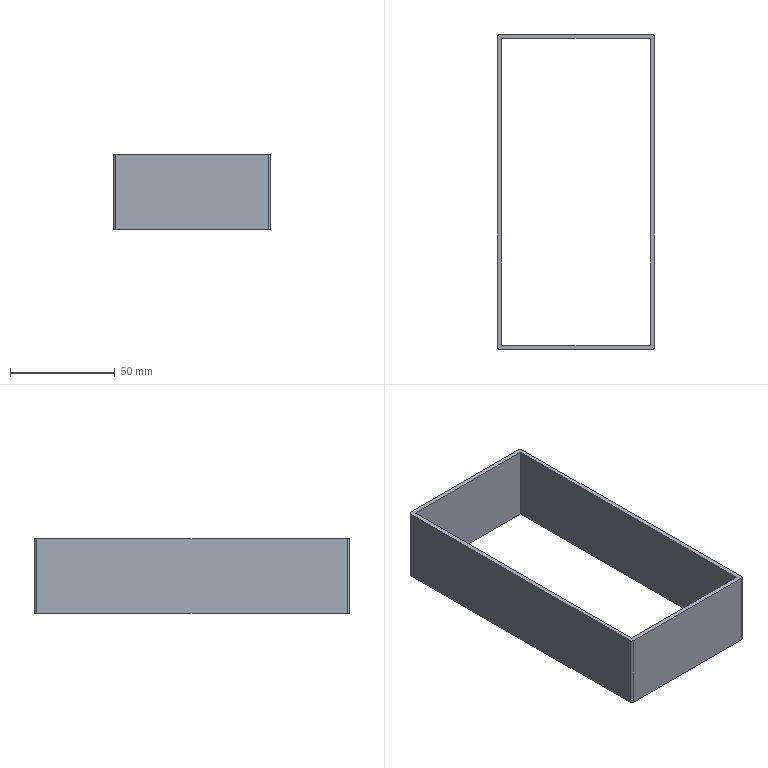Part | STEP file | 11 Timing Pulley盒 EDA50-R-011-BZ^EDA50-R04 (D60N) | 1 solid | 14 faces | box 75 x 150 x 36 mm | volume 31793 mm3 | plane 10 | cylinder 4 | commonest cylinder face diameters 2 x4
STEP:
#1=CARTESIAN_POINT('',(0.,0.,0.));
#2=DIRECTION('',(0.,0.,1.));
#3=DIRECTION('',(1.,0.,0.));
#4=AXIS2_PLACEMENT_3D('',#1,#2,#3);
#5=CARTESIAN_POINT('',(-37.5,113.,18.));
#6=VERTEX_POINT('',#5);
#7=CARTESIAN_POINT('',(-37.5,-35.,18.));
#8=VERTEX_POINT('',#7);
#9=CARTESIAN_POINT('',(-37.5,-36.,18.));
#10=DIRECTION('',(0.,-1.,0.));
#11=VECTOR('',#10,1.);
#12=LINE('',#9,#11);
#13=CARTESIAN_POINT('',(0.,0.,18.));
#14=DIRECTION('',(0.,0.,-1.));
#15=DIRECTION('',(-1.,0.,0.));
#16=AXIS2_PLACEMENT_3D('',#13,#14,#15);
#17=PLANE('',#16);
#18=CARTESIAN_POINT('',(37.5,-36.));
#19=DIRECTION('',(0.,-1.));
#20=VECTOR('',#19,1.);
#21=LINE('',#18,#20);
#22=(GEOMETRIC_REPRESENTATION_CONTEXT(2)PARAMETRIC_REPRESENTATION_CONTEXT()REPRESENTATION_CONTEXT('',''));
#23=DEFINITIONAL_REPRESENTATION('',(#21),#22);
#24=PCURVE('',#17,#23);
#25=CARTESIAN_POINT('',(-37.5,-36.,18.));
#26=DIRECTION('',(1.,0.,0.));
#27=DIRECTION('',(0.,0.,-1.));
#28=AXIS2_PLACEMENT_3D('',#25,#26,#27);
#29=PLANE('',#28);
#30=CARTESIAN_POINT('',(0.,0.));
#31=DIRECTION('',(0.,-1.));
#32=VECTOR('',#31,1.);
#33=LINE('',#30,#32);
#34=(GEOMETRIC_REPRESENTATION_CONTEXT(2)PARAMETRIC_REPRESENTATION_CONTEXT()REPRESENTATION_CONTEXT('',''));
#35=DEFINITIONAL_REPRESENTATION('',(#33),#34);
#36=PCURVE('',#29,#35);
#37=SURFACE_CURVE('',#12,(#24,#36),.PCURVE_S1.);
#38=EDGE_CURVE('',#6,#8,#37,.T.);
#39=ORIENTED_EDGE('',*,*,#38,.T.);
#40=CARTESIAN_POINT('',(-36.5,-36.,18.));
#41=VERTEX_POINT('',#40);
#42=CARTESIAN_POINT('',(-36.5,-35.,18.));
#43=DIRECTION('',(0.,0.,1.));
#44=DIRECTION('',(-1.,0.,0.));
#45=AXIS2_PLACEMENT_3D('',#42,#43,#44);
#46=CIRCLE('',#45,1.);
#47=CARTESIAN_POINT('',(37.5,-35.));
#48=CARTESIAN_POINT('',(37.5,-36.732));
#49=CARTESIAN_POINT('',(36.,-35.866));
#50=CARTESIAN_POINT('',(34.5,-35.));
#51=CARTESIAN_POINT('',(36.,-34.134));
#52=CARTESIAN_POINT('',(37.5,-33.268));
#53=CARTESIAN_POINT('',(37.5,-35.));
#54=(BOUNDED_CURVE()B_SPLINE_CURVE(2,(#47,#48,#49,#50,#51,#52,#53),.UNSPECIFIED.,.T.,.F.)B_SPLINE_CURVE_WITH_KNOTS((1,2,2,2,2,1),(-2.094,0.,2.094,4.189,6.283,8.378),.UNSPECIFIED.)CURVE()GEOMETRIC_REPRESENTATION_ITEM()RATIONAL_B_SPLINE_CURVE((1.,0.5,1.,0.5,1.,0.5,1.))REPRESENTATION_ITEM(''));
#55=(GEOMETRIC_REPRESENTATION_CONTEXT(2)PARAMETRIC_REPRESENTATION_CONTEXT()REPRESENTATION_CONTEXT('',''));
#56=DEFINITIONAL_REPRESENTATION('',(#54),#55);
#57=PCURVE('',#17,#56);
#58=CARTESIAN_POINT('',(-36.5,-35.,18.));
#59=DIRECTION('',(0.,0.,-1.));
#60=DIRECTION('',(-1.,0.,0.));
#61=AXIS2_PLACEMENT_3D('',#58,#59,#60);
#62=CYLINDRICAL_SURFACE('',#61,1.);
#63=CARTESIAN_POINT('',(6.283,0.));
#64=DIRECTION('',(-1.,0.));
#65=VECTOR('',#64,1.);
#66=LINE('',#63,#65);
#67=(GEOMETRIC_REPRESENTATION_CONTEXT(2)PARAMETRIC_REPRESENTATION_CONTEXT()REPRESENTATION_CONTEXT('',''));
#68=DEFINITIONAL_REPRESENTATION('',(#66),#67);
#69=PCURVE('',#62,#68);
#70=SURFACE_CURVE('',#46,(#57,#69),.PCURVE_S1.);
#71=EDGE_CURVE('',#8,#41,#70,.T.);
#72=ORIENTED_EDGE('',*,*,#71,.T.);
#73=CARTESIAN_POINT('',(36.5,-36.,18.));
#74=VERTEX_POINT('',#73);
#75=CARTESIAN_POINT('',(-37.5,-36.,18.));
#76=DIRECTION('',(1.,0.,0.));
#77=VECTOR('',#76,1.);
#78=LINE('',#75,#77);
#79=CARTESIAN_POINT('',(37.5,-36.));
#80=DIRECTION('',(-1.,0.));
#81=VECTOR('',#80,1.);
#82=LINE('',#79,#81);
#83=(GEOMETRIC_REPRESENTATION_CONTEXT(2)PARAMETRIC_REPRESENTATION_CONTEXT()REPRESENTATION_CONTEXT('',''));
#84=DEFINITIONAL_REPRESENTATION('',(#82),#83);
#85=PCURVE('',#17,#84);
#86=CARTESIAN_POINT('',(-37.5,-36.,18.));
#87=DIRECTION('',(0.,1.,0.));
#88=DIRECTION('',(0.,0.,1.));
#89=AXIS2_PLACEMENT_3D('',#86,#87,#88);
#90=PLANE('',#89);
#91=CARTESIAN_POINT('',(0.,0.));
#92=DIRECTION('',(0.,1.));
#93=VECTOR('',#92,1.);
#94=LINE('',#91,#93);
#95=(GEOMETRIC_REPRESENTATION_CONTEXT(2)PARAMETRIC_REPRESENTATION_CONTEXT()REPRESENTATION_CONTEXT('',''));
#96=DEFINITIONAL_REPRESENTATION('',(#94),#95);
#97=PCURVE('',#90,#96);
#98=SURFACE_CURVE('',#78,(#85,#97),.PCURVE_S1.);
#99=EDGE_CURVE('',#41,#74,#98,.T.);
#100=ORIENTED_EDGE('',*,*,#99,.T.);
#101=CARTESIAN_POINT('',(37.5,-35.,18.));
#102=VERTEX_POINT('',#101);
#103=CARTESIAN_POINT('',(36.5,-35.,18.));
#104=DIRECTION('',(0.,0.,1.));
#105=DIRECTION('',(-1.,0.,0.));
#106=AXIS2_PLACEMENT_3D('',#103,#104,#105);
#107=CIRCLE('',#106,1.);
#108=CARTESIAN_POINT('',(-35.5,-35.));
#109=CARTESIAN_POINT('',(-35.5,-36.732));
#110=CARTESIAN_POINT('',(-37.,-35.866));
#111=CARTESIAN_POINT('',(-38.5,-35.));
#112=CARTESIAN_POINT('',(-37.,-34.134));
#113=CARTESIAN_POINT('',(-35.5,-33.268));
#114=CARTESIAN_POINT('',(-35.5,-35.));
#115=(BOUNDED_CURVE()B_SPLINE_CURVE(2,(#108,#109,#110,#111,#112,#113,#114),.UNSPECIFIED.,.T.,.F.)B_SPLINE_CURVE_WITH_KNOTS((1,2,2,2,2,1),(-2.094,0.,2.094,4.189,6.283,8.378),.UNSPECIFIED.)CURVE()GEOMETRIC_REPRESENTATION_ITEM()RATIONAL_B_SPLINE_CURVE((1.,0.5,1.,0.5,1.,0.5,1.))REPRESENTATION_ITEM(''));
#116=(GEOMETRIC_REPRESENTATION_CONTEXT(2)PARAMETRIC_REPRESENTATION_CONTEXT()REPRESENTATION_CONTEXT('',''));
#117=DEFINITIONAL_REPRESENTATION('',(#115),#116);
#118=PCURVE('',#17,#117);
#119=CARTESIAN_POINT('',(36.5,-35.,18.));
#120=DIRECTION('',(0.,0.,-1.));
#121=DIRECTION('',(-1.,0.,0.));
#122=AXIS2_PLACEMENT_3D('',#119,#120,#121);
#123=CYLINDRICAL_SURFACE('',#122,1.);
#124=CARTESIAN_POINT('',(6.283,0.));
#125=DIRECTION('',(-1.,0.));
#126=VECTOR('',#125,1.);
#127=LINE('',#124,#126);
#128=(GEOMETRIC_REPRESENTATION_CONTEXT(2)PARAMETRIC_REPRESENTATION_CONTEXT()REPRESENTATION_CONTEXT('',''));
#129=DEFINITIONAL_REPRESENTATION('',(#127),#128);
#130=PCURVE('',#123,#129);
#131=SURFACE_CURVE('',#107,(#118,#130),.PCURVE_S1.);
#132=EDGE_CURVE('',#74,#102,#131,.T.);
#133=ORIENTED_EDGE('',*,*,#132,.T.);
#134=CARTESIAN_POINT('',(37.5,113.,18.));
#135=VERTEX_POINT('',#134);
#136=CARTESIAN_POINT('',(37.5,-36.,18.));
#137=DIRECTION('',(0.,1.,0.));
#138=VECTOR('',#137,1.);
#139=LINE('',#136,#138);
#140=CARTESIAN_POINT('',(-37.5,-36.));
#141=DIRECTION('',(0.,1.));
#142=VECTOR('',#141,1.);
#143=LINE('',#140,#142);
#144=(GEOMETRIC_REPRESENTATION_CONTEXT(2)PARAMETRIC_REPRESENTATION_CONTEXT()REPRESENTATION_CONTEXT('',''));
#145=DEFINITIONAL_REPRESENTATION('',(#143),#144);
#146=PCURVE('',#17,#145);
#147=CARTESIAN_POINT('',(37.5,-36.,18.));
#148=DIRECTION('',(-1.,0.,0.));
#149=DIRECTION('',(0.,0.,1.));
#150=AXIS2_PLACEMENT_3D('',#147,#148,#149);
#151=PLANE('',#150);
#152=CARTESIAN_POINT('',(0.,0.));
#153=DIRECTION('',(0.,1.));
#154=VECTOR('',#153,1.);
#155=LINE('',#152,#154);
#156=(GEOMETRIC_REPRESENTATION_CONTEXT(2)PARAMETRIC_REPRESENTATION_CONTEXT()REPRESENTATION_CONTEXT('',''));
#157=DEFINITIONAL_REPRESENTATION('',(#155),#156);
#158=PCURVE('',#151,#157);
#159=SURFACE_CURVE('',#139,(#146,#158),.PCURVE_S1.);
#160=EDGE_CURVE('',#102,#135,#159,.T.);
#161=ORIENTED_EDGE('',*,*,#160,.T.);
#162=CARTESIAN_POINT('',(36.5,114.,18.));
#163=VERTEX_POINT('',#162);
#164=CARTESIAN_POINT('',(36.5,113.,18.));
#165=DIRECTION('',(0.,0.,1.));
#166=DIRECTION('',(-1.,0.,0.));
#167=AXIS2_PLACEMENT_3D('',#164,#165,#166);
#168=CIRCLE('',#167,1.);
#169=CARTESIAN_POINT('',(-35.5,113.));
#170=CARTESIAN_POINT('',(-35.5,111.268));
#171=CARTESIAN_POINT('',(-37.,112.134));
#172=CARTESIAN_POINT('',(-38.5,113.));
#173=CARTESIAN_POINT('',(-37.,113.866));
#174=CARTESIAN_POINT('',(-35.5,114.732));
#175=CARTESIAN_POINT('',(-35.5,113.));
#176=(BOUNDED_CURVE()B_SPLINE_CURVE(2,(#169,#170,#171,#172,#173,#174,#175),.UNSPECIFIED.,.T.,.F.)B_SPLINE_CURVE_WITH_KNOTS((1,2,2,2,2,1),(-2.094,0.,2.094,4.189,6.283,8.378),.UNSPECIFIED.)CURVE()GEOMETRIC_REPRESENTATION_ITEM()RATIONAL_B_SPLINE_CURVE((1.,0.5,1.,0.5,1.,0.5,1.))REPRESENTATION_ITEM(''));
#177=(GEOMETRIC_REPRESENTATION_CONTEXT(2)PARAMETRIC_REPRESENTATION_CONTEXT()REPRESENTATION_CONTEXT('',''));
#178=DEFINITIONAL_REPRESENTATION('',(#176),#177);
#179=PCURVE('',#17,#178);
#180=CARTESIAN_POINT('',(36.5,113.,18.));
#181=DIRECTION('',(0.,0.,-1.));
#182=DIRECTION('',(-1.,0.,0.));
#183=AXIS2_PLACEMENT_3D('',#180,#181,#182);
#184=CYLINDRICAL_SURFACE('',#183,1.);
#185=CARTESIAN_POINT('',(6.283,0.));
#186=DIRECTION('',(-1.,0.));
#187=VECTOR('',#186,1.);
#188=LINE('',#185,#187);
#189=(GEOMETRIC_REPRESENTATION_CONTEXT(2)PARAMETRIC_REPRESENTATION_CONTEXT()REPRESENTATION_CONTEXT('',''));
#190=DEFINITIONAL_REPRESENTATION('',(#188),#189);
#191=PCURVE('',#184,#190);
#192=SURFACE_CURVE('',#168,(#179,#191),.PCURVE_S1.);
#193=EDGE_CURVE('',#135,#163,#192,.T.);
#194=ORIENTED_EDGE('',*,*,#193,.T.);
#195=CARTESIAN_POINT('',(-36.5,114.,18.));
#196=VERTEX_POINT('',#195);
#197=CARTESIAN_POINT('',(-37.5,114.,18.));
#198=DIRECTION('',(-1.,0.,0.));
#199=VECTOR('',#198,1.);
#200=LINE('',#197,#199);
#201=CARTESIAN_POINT('',(37.5,114.));
#202=DIRECTION('',(1.,0.));
#203=VECTOR('',#202,1.);
#204=LINE('',#201,#203);
#205=(GEOMETRIC_REPRESENTATION_CONTEXT(2)PARAMETRIC_REPRESENTATION_CONTEXT()REPRESENTATION_CONTEXT('',''));
#206=DEFINITIONAL_REPRESENTATION('',(#204),#205);
#207=PCURVE('',#17,#206);
#208=CARTESIAN_POINT('',(-37.5,114.,18.));
#209=DIRECTION('',(0.,-1.,0.));
#210=DIRECTION('',(0.,0.,-1.));
#211=AXIS2_PLACEMENT_3D('',#208,#209,#210);
#212=PLANE('',#211);
#213=CARTESIAN_POINT('',(0.,0.));
#214=DIRECTION('',(0.,-1.));
#215=VECTOR('',#214,1.);
#216=LINE('',#213,#215);
#217=(GEOMETRIC_REPRESENTATION_CONTEXT(2)PARAMETRIC_REPRESENTATION_CONTEXT()REPRESENTATION_CONTEXT('',''));
#218=DEFINITIONAL_REPRESENTATION('',(#216),#217);
#219=PCURVE('',#212,#218);
#220=SURFACE_CURVE('',#200,(#207,#219),.PCURVE_S1.);
#221=EDGE_CURVE('',#163,#196,#220,.T.);
#222=ORIENTED_EDGE('',*,*,#221,.T.);
#223=CARTESIAN_POINT('',(-36.5,113.,18.));
#224=DIRECTION('',(0.,0.,1.));
#225=DIRECTION('',(-1.,0.,0.));
#226=AXIS2_PLACEMENT_3D('',#223,#224,#225);
#227=CIRCLE('',#226,1.);
#228=CARTESIAN_POINT('',(37.5,113.));
#229=CARTESIAN_POINT('',(37.5,111.268));
#230=CARTESIAN_POINT('',(36.,112.134));
#231=CARTESIAN_POINT('',(34.5,113.));
#232=CARTESIAN_POINT('',(36.,113.866));
#233=CARTESIAN_POINT('',(37.5,114.732));
#234=CARTESIAN_POINT('',(37.5,113.));
#235=(BOUNDED_CURVE()B_SPLINE_CURVE(2,(#228,#229,#230,#231,#232,#233,#234),.UNSPECIFIED.,.T.,.F.)B_SPLINE_CURVE_WITH_KNOTS((1,2,2,2,2,1),(-2.094,0.,2.094,4.189,6.283,8.378),.UNSPECIFIED.)CURVE()GEOMETRIC_REPRESENTATION_ITEM()RATIONAL_B_SPLINE_CURVE((1.,0.5,1.,0.5,1.,0.5,1.))REPRESENTATION_ITEM(''));
#236=(GEOMETRIC_REPRESENTATION_CONTEXT(2)PARAMETRIC_REPRESENTATION_CONTEXT()REPRESENTATION_CONTEXT('',''));
#237=DEFINITIONAL_REPRESENTATION('',(#235),#236);
#238=PCURVE('',#17,#237);
#239=CARTESIAN_POINT('',(-36.5,113.,18.));
#240=DIRECTION('',(0.,0.,-1.));
#241=DIRECTION('',(-1.,0.,0.));
#242=AXIS2_PLACEMENT_3D('',#239,#240,#241);
#243=CYLINDRICAL_SURFACE('',#242,1.);
#244=CARTESIAN_POINT('',(6.283,0.));
#245=DIRECTION('',(-1.,0.));
#246=VECTOR('',#245,1.);
#247=LINE('',#244,#246);
#248=(GEOMETRIC_REPRESENTATION_CONTEXT(2)PARAMETRIC_REPRESENTATION_CONTEXT()REPRESENTATION_CONTEXT('',''));
#249=DEFINITIONAL_REPRESENTATION('',(#247),#248);
#250=PCURVE('',#243,#249);
#251=SURFACE_CURVE('',#227,(#238,#250),.PCURVE_S1.);
#252=EDGE_CURVE('',#196,#6,#251,.T.);
#253=ORIENTED_EDGE('',*,*,#252,.T.);
#254=EDGE_LOOP('',(#39,#72,#100,#133,#161,#194,#222,#253));
#255=FACE_BOUND('',#254,.T.);
#256=CARTESIAN_POINT('',(-35.5,112.,18.));
#257=VERTEX_POINT('',#256);
#258=CARTESIAN_POINT('',(-35.5,-34.,18.));
#259=VERTEX_POINT('',#258);
#260=CARTESIAN_POINT('',(-35.5,-34.,18.));
#261=DIRECTION('',(0.,-1.,0.));
#262=VECTOR('',#261,1.);
#263=LINE('',#260,#262);
#264=CARTESIAN_POINT('',(35.5,-34.));
#265=DIRECTION('',(0.,-1.));
#266=VECTOR('',#265,1.);
#267=LINE('',#264,#266);
#268=(GEOMETRIC_REPRESENTATION_CONTEXT(2)PARAMETRIC_REPRESENTATION_CONTEXT()REPRESENTATION_CONTEXT('',''));
#269=DEFINITIONAL_REPRESENTATION('',(#267),#268);
#270=PCURVE('',#17,#269);
#271=CARTESIAN_POINT('',(-35.5,-34.,18.));
#272=DIRECTION('',(1.,0.,0.));
#273=DIRECTION('',(0.,0.,-1.));
#274=AXIS2_PLACEMENT_3D('',#271,#272,#273);
#275=PLANE('',#274);
#276=CARTESIAN_POINT('',(0.,0.));
#277=DIRECTION('',(0.,-1.));
#278=VECTOR('',#277,1.);
#279=LINE('',#276,#278);
#280=(GEOMETRIC_REPRESENTATION_CONTEXT(2)PARAMETRIC_REPRESENTATION_CONTEXT()REPRESENTATION_CONTEXT('',''));
#281=DEFINITIONAL_REPRESENTATION('',(#279),#280);
#282=PCURVE('',#275,#281);
#283=SURFACE_CURVE('',#263,(#270,#282),.PCURVE_S1.);
#284=EDGE_CURVE('',#257,#259,#283,.T.);
#285=ORIENTED_EDGE('',*,*,#284,.F.);
#286=CARTESIAN_POINT('',(35.5,112.,18.));
#287=VERTEX_POINT('',#286);
#288=CARTESIAN_POINT('',(-35.5,112.,18.));
#289=DIRECTION('',(-1.,0.,0.));
#290=VECTOR('',#289,1.);
#291=LINE('',#288,#290);
#292=CARTESIAN_POINT('',(35.5,112.));
#293=DIRECTION('',(1.,0.));
#294=VECTOR('',#293,1.);
#295=LINE('',#292,#294);
#296=(GEOMETRIC_REPRESENTATION_CONTEXT(2)PARAMETRIC_REPRESENTATION_CONTEXT()REPRESENTATION_CONTEXT('',''));
#297=DEFINITIONAL_REPRESENTATION('',(#295),#296);
#298=PCURVE('',#17,#297);
#299=CARTESIAN_POINT('',(-35.5,112.,18.));
#300=DIRECTION('',(0.,-1.,0.));
#301=DIRECTION('',(0.,0.,-1.));
#302=AXIS2_PLACEMENT_3D('',#299,#300,#301);
#303=PLANE('',#302);
#304=CARTESIAN_POINT('',(0.,0.));
#305=DIRECTION('',(0.,-1.));
#306=VECTOR('',#305,1.);
#307=LINE('',#304,#306);
#308=(GEOMETRIC_REPRESENTATION_CONTEXT(2)PARAMETRIC_REPRESENTATION_CONTEXT()REPRESENTATION_CONTEXT('',''));
#309=DEFINITIONAL_REPRESENTATION('',(#307),#308);
#310=PCURVE('',#303,#309);
#311=SURFACE_CURVE('',#291,(#298,#310),.PCURVE_S1.);
#312=EDGE_CURVE('',#287,#257,#311,.T.);
#313=ORIENTED_EDGE('',*,*,#312,.F.);
#314=CARTESIAN_POINT('',(35.5,-34.,18.));
#315=VERTEX_POINT('',#314);
#316=CARTESIAN_POINT('',(35.5,-34.,18.));
#317=DIRECTION('',(0.,1.,0.));
#318=VECTOR('',#317,1.);
#319=LINE('',#316,#318);
#320=CARTESIAN_POINT('',(-35.5,-34.));
#321=DIRECTION('',(0.,1.));
#322=VECTOR('',#321,1.);
#323=LINE('',#320,#322);
#324=(GEOMETRIC_REPRESENTATION_CONTEXT(2)PARAMETRIC_REPRESENTATION_CONTEXT()REPRESENTATION_CONTEXT('',''));
#325=DEFINITIONAL_REPRESENTATION('',(#323),#324);
#326=PCURVE('',#17,#325);
#327=CARTESIAN_POINT('',(35.5,-34.,18.));
#328=DIRECTION('',(-1.,0.,0.));
#329=DIRECTION('',(0.,0.,1.));
#330=AXIS2_PLACEMENT_3D('',#327,#328,#329);
#331=PLANE('',#330);
#332=CARTESIAN_POINT('',(0.,0.));
#333=DIRECTION('',(0.,1.));
#334=VECTOR('',#333,1.);
#335=LINE('',#332,#334);
#336=(GEOMETRIC_REPRESENTATION_CONTEXT(2)PARAMETRIC_REPRESENTATION_CONTEXT()REPRESENTATION_CONTEXT('',''));
#337=DEFINITIONAL_REPRESENTATION('',(#335),#336);
#338=PCURVE('',#331,#337);
#339=SURFACE_CURVE('',#319,(#326,#338),.PCURVE_S1.);
#340=EDGE_CURVE('',#315,#287,#339,.T.);
#341=ORIENTED_EDGE('',*,*,#340,.F.);
#342=CARTESIAN_POINT('',(-35.5,-34.,18.));
#343=DIRECTION('',(1.,0.,0.));
#344=VECTOR('',#343,1.);
#345=LINE('',#342,#344);
#346=CARTESIAN_POINT('',(35.5,-34.));
#347=DIRECTION('',(-1.,0.));
#348=VECTOR('',#347,1.);
#349=LINE('',#346,#348);
#350=(GEOMETRIC_REPRESENTATION_CONTEXT(2)PARAMETRIC_REPRESENTATION_CONTEXT()REPRESENTATION_CONTEXT('',''));
#351=DEFINITIONAL_REPRESENTATION('',(#349),#350);
#352=PCURVE('',#17,#351);
#353=CARTESIAN_POINT('',(-35.5,-34.,18.));
#354=DIRECTION('',(0.,1.,0.));
#355=DIRECTION('',(0.,0.,1.));
#356=AXIS2_PLACEMENT_3D('',#353,#354,#355);
#357=PLANE('',#356);
#358=CARTESIAN_POINT('',(0.,0.));
#359=DIRECTION('',(0.,1.));
#360=VECTOR('',#359,1.);
#361=LINE('',#358,#360);
#362=(GEOMETRIC_REPRESENTATION_CONTEXT(2)PARAMETRIC_REPRESENTATION_CONTEXT()REPRESENTATION_CONTEXT('',''));
#363=DEFINITIONAL_REPRESENTATION('',(#361),#362);
#364=PCURVE('',#357,#363);
#365=SURFACE_CURVE('',#345,(#352,#364),.PCURVE_S1.);
#366=EDGE_CURVE('',#259,#315,#365,.T.);
#367=ORIENTED_EDGE('',*,*,#366,.F.);
#368=EDGE_LOOP('',(#285,#313,#341,#367));
#369=FACE_BOUND('',#368,.T.);
#370=ADVANCED_FACE('',(#255,#369),#17,.F.);
#371=CARTESIAN_POINT('',(-36.5,-36.,-18.));
#372=VERTEX_POINT('',#371);
#373=CARTESIAN_POINT('',(36.5,-36.,-18.));
#374=VERTEX_POINT('',#373);
#375=CARTESIAN_POINT('',(-37.5,-36.,-18.));
#376=DIRECTION('',(1.,0.,0.));
#377=VECTOR('',#376,1.);
#378=LINE('',#375,#377);
#379=CARTESIAN_POINT('',(0.,0.,-18.));
#380=DIRECTION('',(0.,0.,-1.));
#381=DIRECTION('',(-1.,0.,0.));
#382=AXIS2_PLACEMENT_3D('',#379,#380,#381);
#383=PLANE('',#382);
#384=CARTESIAN_POINT('',(37.5,-36.));
#385=DIRECTION('',(-1.,0.));
#386=VECTOR('',#385,1.);
#387=LINE('',#384,#386);
#388=(GEOMETRIC_REPRESENTATION_CONTEXT(2)PARAMETRIC_REPRESENTATION_CONTEXT()REPRESENTATION_CONTEXT('',''));
#389=DEFINITIONAL_REPRESENTATION('',(#387),#388);
#390=PCURVE('',#383,#389);
#391=CARTESIAN_POINT('',(-36.,0.));
#392=DIRECTION('',(0.,1.));
#393=VECTOR('',#392,1.);
#394=LINE('',#391,#393);
#395=(GEOMETRIC_REPRESENTATION_CONTEXT(2)PARAMETRIC_REPRESENTATION_CONTEXT()REPRESENTATION_CONTEXT('',''));
#396=DEFINITIONAL_REPRESENTATION('',(#394),#395);
#397=PCURVE('',#90,#396);
#398=SURFACE_CURVE('',#378,(#390,#397),.PCURVE_S1.);
#399=EDGE_CURVE('',#372,#374,#398,.T.);
#400=ORIENTED_EDGE('',*,*,#399,.F.);
#401=CARTESIAN_POINT('',(-37.5,-35.,-18.));
#402=VERTEX_POINT('',#401);
#403=CARTESIAN_POINT('',(-36.5,-35.,-18.));
#404=DIRECTION('',(0.,0.,-1.));
#405=DIRECTION('',(-1.,0.,0.));
#406=AXIS2_PLACEMENT_3D('',#403,#404,#405);
#407=CIRCLE('',#406,1.);
#408=CARTESIAN_POINT('',(36.5,-35.));
#409=DIRECTION('',(1.,0.));
#410=AXIS2_PLACEMENT_2D('',#408,#409);
#411=CIRCLE('',#410,1.);
#412=(GEOMETRIC_REPRESENTATION_CONTEXT(2)PARAMETRIC_REPRESENTATION_CONTEXT()REPRESENTATION_CONTEXT('',''));
#413=DEFINITIONAL_REPRESENTATION('',(#411),#412);
#414=PCURVE('',#383,#413);
#415=CARTESIAN_POINT('',(0.,36.));
#416=DIRECTION('',(1.,0.));
#417=VECTOR('',#416,1.);
#418=LINE('',#415,#417);
#419=(GEOMETRIC_REPRESENTATION_CONTEXT(2)PARAMETRIC_REPRESENTATION_CONTEXT()REPRESENTATION_CONTEXT('',''));
#420=DEFINITIONAL_REPRESENTATION('',(#418),#419);
#421=PCURVE('',#62,#420);
#422=SURFACE_CURVE('',#407,(#414,#421),.PCURVE_S1.);
#423=EDGE_CURVE('',#372,#402,#422,.T.);
#424=ORIENTED_EDGE('',*,*,#423,.T.);
#425=CARTESIAN_POINT('',(-37.5,113.,-18.));
#426=VERTEX_POINT('',#425);
#427=CARTESIAN_POINT('',(-37.5,-36.,-18.));
#428=DIRECTION('',(0.,-1.,0.));
#429=VECTOR('',#428,1.);
#430=LINE('',#427,#429);
#431=CARTESIAN_POINT('',(37.5,-36.));
#432=DIRECTION('',(0.,-1.));
#433=VECTOR('',#432,1.);
#434=LINE('',#431,#433);
#435=(GEOMETRIC_REPRESENTATION_CONTEXT(2)PARAMETRIC_REPRESENTATION_CONTEXT()REPRESENTATION_CONTEXT('',''));
#436=DEFINITIONAL_REPRESENTATION('',(#434),#435);
#437=PCURVE('',#383,#436);
#438=CARTESIAN_POINT('',(36.,0.));
#439=DIRECTION('',(0.,-1.));
#440=VECTOR('',#439,1.);
#441=LINE('',#438,#440);
#442=(GEOMETRIC_REPRESENTATION_CONTEXT(2)PARAMETRIC_REPRESENTATION_CONTEXT()REPRESENTATION_CONTEXT('',''));
#443=DEFINITIONAL_REPRESENTATION('',(#441),#442);
#444=PCURVE('',#29,#443);
#445=SURFACE_CURVE('',#430,(#437,#444),.PCURVE_S1.);
#446=EDGE_CURVE('',#426,#402,#445,.T.);
#447=ORIENTED_EDGE('',*,*,#446,.F.);
#448=CARTESIAN_POINT('',(-36.5,114.,-18.));
#449=VERTEX_POINT('',#448);
#450=CARTESIAN_POINT('',(-36.5,113.,-18.));
#451=DIRECTION('',(0.,0.,-1.));
#452=DIRECTION('',(-1.,0.,0.));
#453=AXIS2_PLACEMENT_3D('',#450,#451,#452);
#454=CIRCLE('',#453,1.);
#455=CARTESIAN_POINT('',(36.5,113.));
#456=DIRECTION('',(1.,0.));
#457=AXIS2_PLACEMENT_2D('',#455,#456);
#458=CIRCLE('',#457,1.);
#459=(GEOMETRIC_REPRESENTATION_CONTEXT(2)PARAMETRIC_REPRESENTATION_CONTEXT()REPRESENTATION_CONTEXT('',''));
#460=DEFINITIONAL_REPRESENTATION('',(#458),#459);
#461=PCURVE('',#383,#460);
#462=CARTESIAN_POINT('',(0.,36.));
#463=DIRECTION('',(1.,0.));
#464=VECTOR('',#463,1.);
#465=LINE('',#462,#464);
#466=(GEOMETRIC_REPRESENTATION_CONTEXT(2)PARAMETRIC_REPRESENTATION_CONTEXT()REPRESENTATION_CONTEXT('',''));
#467=DEFINITIONAL_REPRESENTATION('',(#465),#466);
#468=PCURVE('',#243,#467);
#469=SURFACE_CURVE('',#454,(#461,#468),.PCURVE_S1.);
#470=EDGE_CURVE('',#426,#449,#469,.T.);
#471=ORIENTED_EDGE('',*,*,#470,.T.);
#472=CARTESIAN_POINT('',(36.5,114.,-18.));
#473=VERTEX_POINT('',#472);
#474=CARTESIAN_POINT('',(-37.5,114.,-18.));
#475=DIRECTION('',(-1.,0.,0.));
#476=VECTOR('',#475,1.);
#477=LINE('',#474,#476);
#478=CARTESIAN_POINT('',(37.5,114.));
#479=DIRECTION('',(1.,0.));
#480=VECTOR('',#479,1.);
#481=LINE('',#478,#480);
#482=(GEOMETRIC_REPRESENTATION_CONTEXT(2)PARAMETRIC_REPRESENTATION_CONTEXT()REPRESENTATION_CONTEXT('',''));
#483=DEFINITIONAL_REPRESENTATION('',(#481),#482);
#484=PCURVE('',#383,#483);
#485=CARTESIAN_POINT('',(36.,0.));
#486=DIRECTION('',(0.,-1.));
#487=VECTOR('',#486,1.);
#488=LINE('',#485,#487);
#489=(GEOMETRIC_REPRESENTATION_CONTEXT(2)PARAMETRIC_REPRESENTATION_CONTEXT()REPRESENTATION_CONTEXT('',''));
#490=DEFINITIONAL_REPRESENTATION('',(#488),#489);
#491=PCURVE('',#212,#490);
#492=SURFACE_CURVE('',#477,(#484,#491),.PCURVE_S1.);
#493=EDGE_CURVE('',#473,#449,#492,.T.);
#494=ORIENTED_EDGE('',*,*,#493,.F.);
#495=CARTESIAN_POINT('',(37.5,113.,-18.));
#496=VERTEX_POINT('',#495);
#497=CARTESIAN_POINT('',(36.5,113.,-18.));
#498=DIRECTION('',(0.,0.,-1.));
#499=DIRECTION('',(-1.,0.,0.));
#500=AXIS2_PLACEMENT_3D('',#497,#498,#499);
#501=CIRCLE('',#500,1.);
#502=CARTESIAN_POINT('',(-36.5,113.));
#503=DIRECTION('',(1.,0.));
#504=AXIS2_PLACEMENT_2D('',#502,#503);
#505=CIRCLE('',#504,1.);
#506=(GEOMETRIC_REPRESENTATION_CONTEXT(2)PARAMETRIC_REPRESENTATION_CONTEXT()REPRESENTATION_CONTEXT('',''));
#507=DEFINITIONAL_REPRESENTATION('',(#505),#506);
#508=PCURVE('',#383,#507);
#509=CARTESIAN_POINT('',(0.,36.));
#510=DIRECTION('',(1.,0.));
#511=VECTOR('',#510,1.);
#512=LINE('',#509,#511);
#513=(GEOMETRIC_REPRESENTATION_CONTEXT(2)PARAMETRIC_REPRESENTATION_CONTEXT()REPRESENTATION_CONTEXT('',''));
#514=DEFINITIONAL_REPRESENTATION('',(#512),#513);
#515=PCURVE('',#184,#514);
#516=SURFACE_CURVE('',#501,(#508,#515),.PCURVE_S1.);
#517=EDGE_CURVE('',#473,#496,#516,.T.);
#518=ORIENTED_EDGE('',*,*,#517,.T.);
#519=CARTESIAN_POINT('',(37.5,-35.,-18.));
#520=VERTEX_POINT('',#519);
#521=CARTESIAN_POINT('',(37.5,-36.,-18.));
#522=DIRECTION('',(0.,1.,0.));
#523=VECTOR('',#522,1.);
#524=LINE('',#521,#523);
#525=CARTESIAN_POINT('',(-37.5,-36.));
#526=DIRECTION('',(0.,1.));
#527=VECTOR('',#526,1.);
#528=LINE('',#525,#527);
#529=(GEOMETRIC_REPRESENTATION_CONTEXT(2)PARAMETRIC_REPRESENTATION_CONTEXT()REPRESENTATION_CONTEXT('',''));
#530=DEFINITIONAL_REPRESENTATION('',(#528),#529);
#531=PCURVE('',#383,#530);
#532=CARTESIAN_POINT('',(-36.,0.));
#533=DIRECTION('',(0.,1.));
#534=VECTOR('',#533,1.);
#535=LINE('',#532,#534);
#536=(GEOMETRIC_REPRESENTATION_CONTEXT(2)PARAMETRIC_REPRESENTATION_CONTEXT()REPRESENTATION_CONTEXT('',''));
#537=DEFINITIONAL_REPRESENTATION('',(#535),#536);
#538=PCURVE('',#151,#537);
#539=SURFACE_CURVE('',#524,(#531,#538),.PCURVE_S1.);
#540=EDGE_CURVE('',#520,#496,#539,.T.);
#541=ORIENTED_EDGE('',*,*,#540,.F.);
#542=CARTESIAN_POINT('',(36.5,-35.,-18.));
#543=DIRECTION('',(0.,0.,-1.));
#544=DIRECTION('',(-1.,0.,0.));
#545=AXIS2_PLACEMENT_3D('',#542,#543,#544);
#546=CIRCLE('',#545,1.);
#547=CARTESIAN_POINT('',(-36.5,-35.));
#548=DIRECTION('',(1.,0.));
#549=AXIS2_PLACEMENT_2D('',#547,#548);
#550=CIRCLE('',#549,1.);
#551=(GEOMETRIC_REPRESENTATION_CONTEXT(2)PARAMETRIC_REPRESENTATION_CONTEXT()REPRESENTATION_CONTEXT('',''));
#552=DEFINITIONAL_REPRESENTATION('',(#550),#551);
#553=PCURVE('',#383,#552);
#554=CARTESIAN_POINT('',(0.,36.));
#555=DIRECTION('',(1.,0.));
#556=VECTOR('',#555,1.);
#557=LINE('',#554,#556);
#558=(GEOMETRIC_REPRESENTATION_CONTEXT(2)PARAMETRIC_REPRESENTATION_CONTEXT()REPRESENTATION_CONTEXT('',''));
#559=DEFINITIONAL_REPRESENTATION('',(#557),#558);
#560=PCURVE('',#123,#559);
#561=SURFACE_CURVE('',#546,(#553,#560),.PCURVE_S1.);
#562=EDGE_CURVE('',#520,#374,#561,.T.);
#563=ORIENTED_EDGE('',*,*,#562,.T.);
#564=EDGE_LOOP('',(#400,#424,#447,#471,#494,#518,#541,#563));
#565=FACE_BOUND('',#564,.T.);
#566=CARTESIAN_POINT('',(35.5,112.,-18.));
#567=VERTEX_POINT('',#566);
#568=CARTESIAN_POINT('',(-35.5,112.,-18.));
#569=VERTEX_POINT('',#568);
#570=CARTESIAN_POINT('',(-35.5,112.,-18.));
#571=DIRECTION('',(-1.,0.,0.));
#572=VECTOR('',#571,1.);
#573=LINE('',#570,#572);
#574=CARTESIAN_POINT('',(35.5,112.));
#575=DIRECTION('',(1.,0.));
#576=VECTOR('',#575,1.);
#577=LINE('',#574,#576);
#578=(GEOMETRIC_REPRESENTATION_CONTEXT(2)PARAMETRIC_REPRESENTATION_CONTEXT()REPRESENTATION_CONTEXT('',''));
#579=DEFINITIONAL_REPRESENTATION('',(#577),#578);
#580=PCURVE('',#383,#579);
#581=CARTESIAN_POINT('',(36.,0.));
#582=DIRECTION('',(0.,-1.));
#583=VECTOR('',#582,1.);
#584=LINE('',#581,#583);
#585=(GEOMETRIC_REPRESENTATION_CONTEXT(2)PARAMETRIC_REPRESENTATION_CONTEXT()REPRESENTATION_CONTEXT('',''));
#586=DEFINITIONAL_REPRESENTATION('',(#584),#585);
#587=PCURVE('',#303,#586);
#588=SURFACE_CURVE('',#573,(#580,#587),.PCURVE_S1.);
#589=EDGE_CURVE('',#567,#569,#588,.T.);
#590=ORIENTED_EDGE('',*,*,#589,.T.);
#591=CARTESIAN_POINT('',(-35.5,-34.,-18.));
#592=VERTEX_POINT('',#591);
#593=CARTESIAN_POINT('',(-35.5,-34.,-18.));
#594=DIRECTION('',(0.,-1.,0.));
#595=VECTOR('',#594,1.);
#596=LINE('',#593,#595);
#597=CARTESIAN_POINT('',(35.5,-34.));
#598=DIRECTION('',(0.,-1.));
#599=VECTOR('',#598,1.);
#600=LINE('',#597,#599);
#601=(GEOMETRIC_REPRESENTATION_CONTEXT(2)PARAMETRIC_REPRESENTATION_CONTEXT()REPRESENTATION_CONTEXT('',''));
#602=DEFINITIONAL_REPRESENTATION('',(#600),#601);
#603=PCURVE('',#383,#602);
#604=CARTESIAN_POINT('',(36.,0.));
#605=DIRECTION('',(0.,-1.));
#606=VECTOR('',#605,1.);
#607=LINE('',#604,#606);
#608=(GEOMETRIC_REPRESENTATION_CONTEXT(2)PARAMETRIC_REPRESENTATION_CONTEXT()REPRESENTATION_CONTEXT('',''));
#609=DEFINITIONAL_REPRESENTATION('',(#607),#608);
#610=PCURVE('',#275,#609);
#611=SURFACE_CURVE('',#596,(#603,#610),.PCURVE_S1.);
#612=EDGE_CURVE('',#569,#592,#611,.T.);
#613=ORIENTED_EDGE('',*,*,#612,.T.);
#614=CARTESIAN_POINT('',(35.5,-34.,-18.));
#615=VERTEX_POINT('',#614);
#616=CARTESIAN_POINT('',(-35.5,-34.,-18.));
#617=DIRECTION('',(1.,0.,0.));
#618=VECTOR('',#617,1.);
#619=LINE('',#616,#618);
#620=CARTESIAN_POINT('',(35.5,-34.));
#621=DIRECTION('',(-1.,0.));
#622=VECTOR('',#621,1.);
#623=LINE('',#620,#622);
#624=(GEOMETRIC_REPRESENTATION_CONTEXT(2)PARAMETRIC_REPRESENTATION_CONTEXT()REPRESENTATION_CONTEXT('',''));
#625=DEFINITIONAL_REPRESENTATION('',(#623),#624);
#626=PCURVE('',#383,#625);
#627=CARTESIAN_POINT('',(-36.,0.));
#628=DIRECTION('',(0.,1.));
#629=VECTOR('',#628,1.);
#630=LINE('',#627,#629);
#631=(GEOMETRIC_REPRESENTATION_CONTEXT(2)PARAMETRIC_REPRESENTATION_CONTEXT()REPRESENTATION_CONTEXT('',''));
#632=DEFINITIONAL_REPRESENTATION('',(#630),#631);
#633=PCURVE('',#357,#632);
#634=SURFACE_CURVE('',#619,(#626,#633),.PCURVE_S1.);
#635=EDGE_CURVE('',#592,#615,#634,.T.);
#636=ORIENTED_EDGE('',*,*,#635,.T.);
#637=CARTESIAN_POINT('',(35.5,-34.,-18.));
#638=DIRECTION('',(0.,1.,0.));
#639=VECTOR('',#638,1.);
#640=LINE('',#637,#639);
#641=CARTESIAN_POINT('',(-35.5,-34.));
#642=DIRECTION('',(0.,1.));
#643=VECTOR('',#642,1.);
#644=LINE('',#641,#643);
#645=(GEOMETRIC_REPRESENTATION_CONTEXT(2)PARAMETRIC_REPRESENTATION_CONTEXT()REPRESENTATION_CONTEXT('',''));
#646=DEFINITIONAL_REPRESENTATION('',(#644),#645);
#647=PCURVE('',#383,#646);
#648=CARTESIAN_POINT('',(-36.,0.));
#649=DIRECTION('',(0.,1.));
#650=VECTOR('',#649,1.);
#651=LINE('',#648,#650);
#652=(GEOMETRIC_REPRESENTATION_CONTEXT(2)PARAMETRIC_REPRESENTATION_CONTEXT()REPRESENTATION_CONTEXT('',''));
#653=DEFINITIONAL_REPRESENTATION('',(#651),#652);
#654=PCURVE('',#331,#653);
#655=SURFACE_CURVE('',#640,(#647,#654),.PCURVE_S1.);
#656=EDGE_CURVE('',#615,#567,#655,.T.);
#657=ORIENTED_EDGE('',*,*,#656,.T.);
#658=EDGE_LOOP('',(#590,#613,#636,#657));
#659=FACE_BOUND('',#658,.T.);
#660=ADVANCED_FACE('',(#565,#659),#383,.T.);
#661=ORIENTED_EDGE('',*,*,#446,.T.);
#662=CARTESIAN_POINT('',(-37.5,-35.,18.));
#663=DIRECTION('',(0.,0.,1.));
#664=VECTOR('',#663,1.);
#665=LINE('',#662,#664);
#666=CARTESIAN_POINT('',(0.,1.));
#667=DIRECTION('',(-1.,0.));
#668=VECTOR('',#667,1.);
#669=LINE('',#666,#668);
#670=(GEOMETRIC_REPRESENTATION_CONTEXT(2)PARAMETRIC_REPRESENTATION_CONTEXT()REPRESENTATION_CONTEXT('',''));
#671=DEFINITIONAL_REPRESENTATION('',(#669),#670);
#672=PCURVE('',#29,#671);
#673=CARTESIAN_POINT('',(6.283,0.));
#674=DIRECTION('',(0.,-1.));
#675=VECTOR('',#674,1.);
#676=LINE('',#673,#675);
#677=(GEOMETRIC_REPRESENTATION_CONTEXT(2)PARAMETRIC_REPRESENTATION_CONTEXT()REPRESENTATION_CONTEXT('',''));
#678=DEFINITIONAL_REPRESENTATION('',(#676),#677);
#679=PCURVE('',#62,#678);
#680=SURFACE_CURVE('',#665,(#672,#679),.PCURVE_S1.);
#681=EDGE_CURVE('',#402,#8,#680,.T.);
#682=ORIENTED_EDGE('',*,*,#681,.T.);
#683=ORIENTED_EDGE('',*,*,#38,.F.);
#684=CARTESIAN_POINT('',(-37.5,113.,18.));
#685=DIRECTION('',(0.,0.,-1.));
#686=VECTOR('',#685,1.);
#687=LINE('',#684,#686);
#688=CARTESIAN_POINT('',(0.,149.));
#689=DIRECTION('',(1.,0.));
#690=VECTOR('',#689,1.);
#691=LINE('',#688,#690);
#692=(GEOMETRIC_REPRESENTATION_CONTEXT(2)PARAMETRIC_REPRESENTATION_CONTEXT()REPRESENTATION_CONTEXT('',''));
#693=DEFINITIONAL_REPRESENTATION('',(#691),#692);
#694=PCURVE('',#29,#693);
#695=CARTESIAN_POINT('',(0.,0.));
#696=DIRECTION('',(0.,1.));
#697=VECTOR('',#696,1.);
#698=LINE('',#695,#697);
#699=(GEOMETRIC_REPRESENTATION_CONTEXT(2)PARAMETRIC_REPRESENTATION_CONTEXT()REPRESENTATION_CONTEXT('',''));
#700=DEFINITIONAL_REPRESENTATION('',(#698),#699);
#701=PCURVE('',#243,#700);
#702=SURFACE_CURVE('',#687,(#694,#701),.PCURVE_S1.);
#703=EDGE_CURVE('',#6,#426,#702,.T.);
#704=ORIENTED_EDGE('',*,*,#703,.T.);
#705=EDGE_LOOP('',(#661,#682,#683,#704));
#706=FACE_BOUND('',#705,.T.);
#707=ADVANCED_FACE('',(#706),#29,.F.);
#708=ORIENTED_EDGE('',*,*,#99,.F.);
#709=CARTESIAN_POINT('',(-36.5,-36.,18.));
#710=DIRECTION('',(0.,0.,-1.));
#711=VECTOR('',#710,1.);
#712=LINE('',#709,#711);
#713=CARTESIAN_POINT('',(0.,1.));
#714=DIRECTION('',(-1.,0.));
#715=VECTOR('',#714,1.);
#716=LINE('',#713,#715);
#717=(GEOMETRIC_REPRESENTATION_CONTEXT(2)PARAMETRIC_REPRESENTATION_CONTEXT()REPRESENTATION_CONTEXT('',''));
#718=DEFINITIONAL_REPRESENTATION('',(#716),#717);
#719=PCURVE('',#90,#718);
#720=CARTESIAN_POINT('',(4.712,0.));
#721=DIRECTION('',(0.,1.));
#722=VECTOR('',#721,1.);
#723=LINE('',#720,#722);
#724=(GEOMETRIC_REPRESENTATION_CONTEXT(2)PARAMETRIC_REPRESENTATION_CONTEXT()REPRESENTATION_CONTEXT('',''));
#725=DEFINITIONAL_REPRESENTATION('',(#723),#724);
#726=PCURVE('',#62,#725);
#727=SURFACE_CURVE('',#712,(#719,#726),.PCURVE_S1.);
#728=EDGE_CURVE('',#41,#372,#727,.T.);
#729=ORIENTED_EDGE('',*,*,#728,.T.);
#730=ORIENTED_EDGE('',*,*,#399,.T.);
#731=CARTESIAN_POINT('',(36.5,-36.,18.));
#732=DIRECTION('',(0.,0.,1.));
#733=VECTOR('',#732,1.);
#734=LINE('',#731,#733);
#735=CARTESIAN_POINT('',(0.,74.));
#736=DIRECTION('',(1.,0.));
#737=VECTOR('',#736,1.);
#738=LINE('',#735,#737);
#739=(GEOMETRIC_REPRESENTATION_CONTEXT(2)PARAMETRIC_REPRESENTATION_CONTEXT()REPRESENTATION_CONTEXT('',''));
#740=DEFINITIONAL_REPRESENTATION('',(#738),#739);
#741=PCURVE('',#90,#740);
#742=CARTESIAN_POINT('',(4.712,0.));
#743=DIRECTION('',(0.,-1.));
#744=VECTOR('',#743,1.);
#745=LINE('',#742,#744);
#746=(GEOMETRIC_REPRESENTATION_CONTEXT(2)PARAMETRIC_REPRESENTATION_CONTEXT()REPRESENTATION_CONTEXT('',''));
#747=DEFINITIONAL_REPRESENTATION('',(#745),#746);
#748=PCURVE('',#123,#747);
#749=SURFACE_CURVE('',#734,(#741,#748),.PCURVE_S1.);
#750=EDGE_CURVE('',#374,#74,#749,.T.);
#751=ORIENTED_EDGE('',*,*,#750,.T.);
#752=EDGE_LOOP('',(#708,#729,#730,#751));
#753=FACE_BOUND('',#752,.T.);
#754=ADVANCED_FACE('',(#753),#90,.F.);
#755=ORIENTED_EDGE('',*,*,#160,.F.);
#756=CARTESIAN_POINT('',(37.5,-35.,18.));
#757=DIRECTION('',(0.,0.,-1.));
#758=VECTOR('',#757,1.);
#759=LINE('',#756,#758);
#760=CARTESIAN_POINT('',(0.,1.));
#761=DIRECTION('',(-1.,0.));
#762=VECTOR('',#761,1.);
#763=LINE('',#760,#762);
#764=(GEOMETRIC_REPRESENTATION_CONTEXT(2)PARAMETRIC_REPRESENTATION_CONTEXT()REPRESENTATION_CONTEXT('',''));
#765=DEFINITIONAL_REPRESENTATION('',(#763),#764);
#766=PCURVE('',#151,#765);
#767=CARTESIAN_POINT('',(3.142,0.));
#768=DIRECTION('',(0.,1.));
#769=VECTOR('',#768,1.);
#770=LINE('',#767,#769);
#771=(GEOMETRIC_REPRESENTATION_CONTEXT(2)PARAMETRIC_REPRESENTATION_CONTEXT()REPRESENTATION_CONTEXT('',''));
#772=DEFINITIONAL_REPRESENTATION('',(#770),#771);
#773=PCURVE('',#123,#772);
#774=SURFACE_CURVE('',#759,(#766,#773),.PCURVE_S1.);
#775=EDGE_CURVE('',#102,#520,#774,.T.);
#776=ORIENTED_EDGE('',*,*,#775,.T.);
#777=ORIENTED_EDGE('',*,*,#540,.T.);
#778=CARTESIAN_POINT('',(37.5,113.,18.));
#779=DIRECTION('',(0.,0.,1.));
#780=VECTOR('',#779,1.);
#781=LINE('',#778,#780);
#782=CARTESIAN_POINT('',(0.,149.));
#783=DIRECTION('',(1.,0.));
#784=VECTOR('',#783,1.);
#785=LINE('',#782,#784);
#786=(GEOMETRIC_REPRESENTATION_CONTEXT(2)PARAMETRIC_REPRESENTATION_CONTEXT()REPRESENTATION_CONTEXT('',''));
#787=DEFINITIONAL_REPRESENTATION('',(#785),#786);
#788=PCURVE('',#151,#787);
#789=CARTESIAN_POINT('',(3.142,0.));
#790=DIRECTION('',(0.,-1.));
#791=VECTOR('',#790,1.);
#792=LINE('',#789,#791);
#793=(GEOMETRIC_REPRESENTATION_CONTEXT(2)PARAMETRIC_REPRESENTATION_CONTEXT()REPRESENTATION_CONTEXT('',''));
#794=DEFINITIONAL_REPRESENTATION('',(#792),#793);
#795=PCURVE('',#184,#794);
#796=SURFACE_CURVE('',#781,(#788,#795),.PCURVE_S1.);
#797=EDGE_CURVE('',#496,#135,#796,.T.);
#798=ORIENTED_EDGE('',*,*,#797,.T.);
#799=EDGE_LOOP('',(#755,#776,#777,#798));
#800=FACE_BOUND('',#799,.T.);
#801=ADVANCED_FACE('',(#800),#151,.F.);
#802=ORIENTED_EDGE('',*,*,#493,.T.);
#803=CARTESIAN_POINT('',(-36.5,114.,18.));
#804=DIRECTION('',(0.,0.,1.));
#805=VECTOR('',#804,1.);
#806=LINE('',#803,#805);
#807=CARTESIAN_POINT('',(0.,1.));
#808=DIRECTION('',(-1.,0.));
#809=VECTOR('',#808,1.);
#810=LINE('',#807,#809);
#811=(GEOMETRIC_REPRESENTATION_CONTEXT(2)PARAMETRIC_REPRESENTATION_CONTEXT()REPRESENTATION_CONTEXT('',''));
#812=DEFINITIONAL_REPRESENTATION('',(#810),#811);
#813=PCURVE('',#212,#812);
#814=CARTESIAN_POINT('',(1.571,0.));
#815=DIRECTION('',(0.,-1.));
#816=VECTOR('',#815,1.);
#817=LINE('',#814,#816);
#818=(GEOMETRIC_REPRESENTATION_CONTEXT(2)PARAMETRIC_REPRESENTATION_CONTEXT()REPRESENTATION_CONTEXT('',''));
#819=DEFINITIONAL_REPRESENTATION('',(#817),#818);
#820=PCURVE('',#243,#819);
#821=SURFACE_CURVE('',#806,(#813,#820),.PCURVE_S1.);
#822=EDGE_CURVE('',#449,#196,#821,.T.);
#823=ORIENTED_EDGE('',*,*,#822,.T.);
#824=ORIENTED_EDGE('',*,*,#221,.F.);
#825=CARTESIAN_POINT('',(36.5,114.,18.));
#826=DIRECTION('',(0.,0.,-1.));
#827=VECTOR('',#826,1.);
#828=LINE('',#825,#827);
#829=CARTESIAN_POINT('',(0.,74.));
#830=DIRECTION('',(1.,0.));
#831=VECTOR('',#830,1.);
#832=LINE('',#829,#831);
#833=(GEOMETRIC_REPRESENTATION_CONTEXT(2)PARAMETRIC_REPRESENTATION_CONTEXT()REPRESENTATION_CONTEXT('',''));
#834=DEFINITIONAL_REPRESENTATION('',(#832),#833);
#835=PCURVE('',#212,#834);
#836=CARTESIAN_POINT('',(1.571,0.));
#837=DIRECTION('',(0.,1.));
#838=VECTOR('',#837,1.);
#839=LINE('',#836,#838);
#840=(GEOMETRIC_REPRESENTATION_CONTEXT(2)PARAMETRIC_REPRESENTATION_CONTEXT()REPRESENTATION_CONTEXT('',''));
#841=DEFINITIONAL_REPRESENTATION('',(#839),#840);
#842=PCURVE('',#184,#841);
#843=SURFACE_CURVE('',#828,(#835,#842),.PCURVE_S1.);
#844=EDGE_CURVE('',#163,#473,#843,.T.);
#845=ORIENTED_EDGE('',*,*,#844,.T.);
#846=EDGE_LOOP('',(#802,#823,#824,#845));
#847=FACE_BOUND('',#846,.T.);
#848=ADVANCED_FACE('',(#847),#212,.F.);
#849=ORIENTED_EDGE('',*,*,#612,.F.);
#850=CARTESIAN_POINT('',(-35.5,112.,18.));
#851=DIRECTION('',(0.,0.,-1.));
#852=VECTOR('',#851,1.);
#853=LINE('',#850,#852);
#854=CARTESIAN_POINT('',(0.,146.));
#855=DIRECTION('',(1.,0.));
#856=VECTOR('',#855,1.);
#857=LINE('',#854,#856);
#858=(GEOMETRIC_REPRESENTATION_CONTEXT(2)PARAMETRIC_REPRESENTATION_CONTEXT()REPRESENTATION_CONTEXT('',''));
#859=DEFINITIONAL_REPRESENTATION('',(#857),#858);
#860=PCURVE('',#275,#859);
#861=CARTESIAN_POINT('',(0.,0.));
#862=DIRECTION('',(1.,0.));
#863=VECTOR('',#862,1.);
#864=LINE('',#861,#863);
#865=(GEOMETRIC_REPRESENTATION_CONTEXT(2)PARAMETRIC_REPRESENTATION_CONTEXT()REPRESENTATION_CONTEXT('',''));
#866=DEFINITIONAL_REPRESENTATION('',(#864),#865);
#867=PCURVE('',#303,#866);
#868=SURFACE_CURVE('',#853,(#860,#867),.PCURVE_S1.);
#869=EDGE_CURVE('',#257,#569,#868,.T.);
#870=ORIENTED_EDGE('',*,*,#869,.F.);
#871=ORIENTED_EDGE('',*,*,#284,.T.);
#872=CARTESIAN_POINT('',(-35.5,-34.,18.));
#873=DIRECTION('',(0.,0.,-1.));
#874=VECTOR('',#873,1.);
#875=LINE('',#872,#874);
#876=CARTESIAN_POINT('',(0.,0.));
#877=DIRECTION('',(1.,0.));
#878=VECTOR('',#877,1.);
#879=LINE('',#876,#878);
#880=(GEOMETRIC_REPRESENTATION_CONTEXT(2)PARAMETRIC_REPRESENTATION_CONTEXT()REPRESENTATION_CONTEXT('',''));
#881=DEFINITIONAL_REPRESENTATION('',(#879),#880);
#882=PCURVE('',#275,#881);
#883=CARTESIAN_POINT('',(0.,0.));
#884=DIRECTION('',(-1.,0.));
#885=VECTOR('',#884,1.);
#886=LINE('',#883,#885);
#887=(GEOMETRIC_REPRESENTATION_CONTEXT(2)PARAMETRIC_REPRESENTATION_CONTEXT()REPRESENTATION_CONTEXT('',''));
#888=DEFINITIONAL_REPRESENTATION('',(#886),#887);
#889=PCURVE('',#357,#888);
#890=SURFACE_CURVE('',#875,(#882,#889),.PCURVE_S1.);
#891=EDGE_CURVE('',#259,#592,#890,.T.);
#892=ORIENTED_EDGE('',*,*,#891,.T.);
#893=EDGE_LOOP('',(#849,#870,#871,#892));
#894=FACE_BOUND('',#893,.T.);
#895=ADVANCED_FACE('',(#894),#275,.T.);
#896=ORIENTED_EDGE('',*,*,#635,.F.);
#897=ORIENTED_EDGE('',*,*,#891,.F.);
#898=ORIENTED_EDGE('',*,*,#366,.T.);
#899=CARTESIAN_POINT('',(35.5,-34.,18.));
#900=DIRECTION('',(0.,0.,-1.));
#901=VECTOR('',#900,1.);
#902=LINE('',#899,#901);
#903=CARTESIAN_POINT('',(0.,71.));
#904=DIRECTION('',(-1.,0.));
#905=VECTOR('',#904,1.);
#906=LINE('',#903,#905);
#907=(GEOMETRIC_REPRESENTATION_CONTEXT(2)PARAMETRIC_REPRESENTATION_CONTEXT()REPRESENTATION_CONTEXT('',''));
#908=DEFINITIONAL_REPRESENTATION('',(#906),#907);
#909=PCURVE('',#357,#908);
#910=CARTESIAN_POINT('',(0.,0.));
#911=DIRECTION('',(-1.,0.));
#912=VECTOR('',#911,1.);
#913=LINE('',#910,#912);
#914=(GEOMETRIC_REPRESENTATION_CONTEXT(2)PARAMETRIC_REPRESENTATION_CONTEXT()REPRESENTATION_CONTEXT('',''));
#915=DEFINITIONAL_REPRESENTATION('',(#913),#914);
#916=PCURVE('',#331,#915);
#917=SURFACE_CURVE('',#902,(#909,#916),.PCURVE_S1.);
#918=EDGE_CURVE('',#315,#615,#917,.T.);
#919=ORIENTED_EDGE('',*,*,#918,.T.);
#920=EDGE_LOOP('',(#896,#897,#898,#919));
#921=FACE_BOUND('',#920,.T.);
#922=ADVANCED_FACE('',(#921),#357,.T.);
#923=ORIENTED_EDGE('',*,*,#656,.F.);
#924=ORIENTED_EDGE('',*,*,#918,.F.);
#925=ORIENTED_EDGE('',*,*,#340,.T.);
#926=CARTESIAN_POINT('',(35.5,112.,18.));
#927=DIRECTION('',(0.,0.,-1.));
#928=VECTOR('',#927,1.);
#929=LINE('',#926,#928);
#930=CARTESIAN_POINT('',(0.,146.));
#931=DIRECTION('',(-1.,0.));
#932=VECTOR('',#931,1.);
#933=LINE('',#930,#932);
#934=(GEOMETRIC_REPRESENTATION_CONTEXT(2)PARAMETRIC_REPRESENTATION_CONTEXT()REPRESENTATION_CONTEXT('',''));
#935=DEFINITIONAL_REPRESENTATION('',(#933),#934);
#936=PCURVE('',#331,#935);
#937=CARTESIAN_POINT('',(0.,71.));
#938=DIRECTION('',(1.,0.));
#939=VECTOR('',#938,1.);
#940=LINE('',#937,#939);
#941=(GEOMETRIC_REPRESENTATION_CONTEXT(2)PARAMETRIC_REPRESENTATION_CONTEXT()REPRESENTATION_CONTEXT('',''));
#942=DEFINITIONAL_REPRESENTATION('',(#940),#941);
#943=PCURVE('',#303,#942);
#944=SURFACE_CURVE('',#929,(#936,#943),.PCURVE_S1.);
#945=EDGE_CURVE('',#287,#567,#944,.T.);
#946=ORIENTED_EDGE('',*,*,#945,.T.);
#947=EDGE_LOOP('',(#923,#924,#925,#946));
#948=FACE_BOUND('',#947,.T.);
#949=ADVANCED_FACE('',(#948),#331,.T.);
#950=ORIENTED_EDGE('',*,*,#589,.F.);
#951=ORIENTED_EDGE('',*,*,#945,.F.);
#952=ORIENTED_EDGE('',*,*,#312,.T.);
#953=ORIENTED_EDGE('',*,*,#869,.T.);
#954=EDGE_LOOP('',(#950,#951,#952,#953));
#955=FACE_BOUND('',#954,.T.);
#956=ADVANCED_FACE('',(#955),#303,.T.);
#957=ORIENTED_EDGE('',*,*,#71,.F.);
#958=ORIENTED_EDGE('',*,*,#681,.F.);
#959=ORIENTED_EDGE('',*,*,#423,.F.);
#960=ORIENTED_EDGE('',*,*,#728,.F.);
#961=EDGE_LOOP('',(#957,#958,#959,#960));
#962=FACE_BOUND('',#961,.T.);
#963=ADVANCED_FACE('',(#962),#62,.T.);
#964=ORIENTED_EDGE('',*,*,#132,.F.);
#965=ORIENTED_EDGE('',*,*,#750,.F.);
#966=ORIENTED_EDGE('',*,*,#562,.F.);
#967=ORIENTED_EDGE('',*,*,#775,.F.);
#968=EDGE_LOOP('',(#964,#965,#966,#967));
#969=FACE_BOUND('',#968,.T.);
#970=ADVANCED_FACE('',(#969),#123,.T.);
#971=ORIENTED_EDGE('',*,*,#252,.F.);
#972=ORIENTED_EDGE('',*,*,#822,.F.);
#973=ORIENTED_EDGE('',*,*,#470,.F.);
#974=ORIENTED_EDGE('',*,*,#703,.F.);
#975=EDGE_LOOP('',(#971,#972,#973,#974));
#976=FACE_BOUND('',#975,.T.);
#977=ADVANCED_FACE('',(#976),#243,.T.);
#978=ORIENTED_EDGE('',*,*,#193,.F.);
#979=ORIENTED_EDGE('',*,*,#797,.F.);
#980=ORIENTED_EDGE('',*,*,#517,.F.);
#981=ORIENTED_EDGE('',*,*,#844,.F.);
#982=EDGE_LOOP('',(#978,#979,#980,#981));
#983=FACE_BOUND('',#982,.T.);
#984=ADVANCED_FACE('',(#983),#184,.T.);
#985=CLOSED_SHELL('',(#370,#660,#707,#754,#801,#848,#895,#922,#949,#956,#963,#970,#977,#984));
#986=MANIFOLD_SOLID_BREP('',#985);
#987=(LENGTH_UNIT()NAMED_UNIT(*)SI_UNIT(.MILLI.,.METRE.));
#988=UNCERTAINTY_MEASURE_WITH_UNIT(LENGTH_MEASURE(0.0000001),#987,'','');
#989=(NAMED_UNIT(*)PLANE_ANGLE_UNIT()SI_UNIT($,.RADIAN.));
#990=(NAMED_UNIT(*)SI_UNIT($,.STERADIAN.)SOLID_ANGLE_UNIT());
#991=(GEOMETRIC_REPRESENTATION_CONTEXT(3)GLOBAL_UNCERTAINTY_ASSIGNED_CONTEXT((#988))GLOBAL_UNIT_ASSIGNED_CONTEXT((#987,#989,#990))REPRESENTATION_CONTEXT('',''));
#992=ADVANCED_BREP_SHAPE_REPRESENTATION('',(#4,#986),#991);